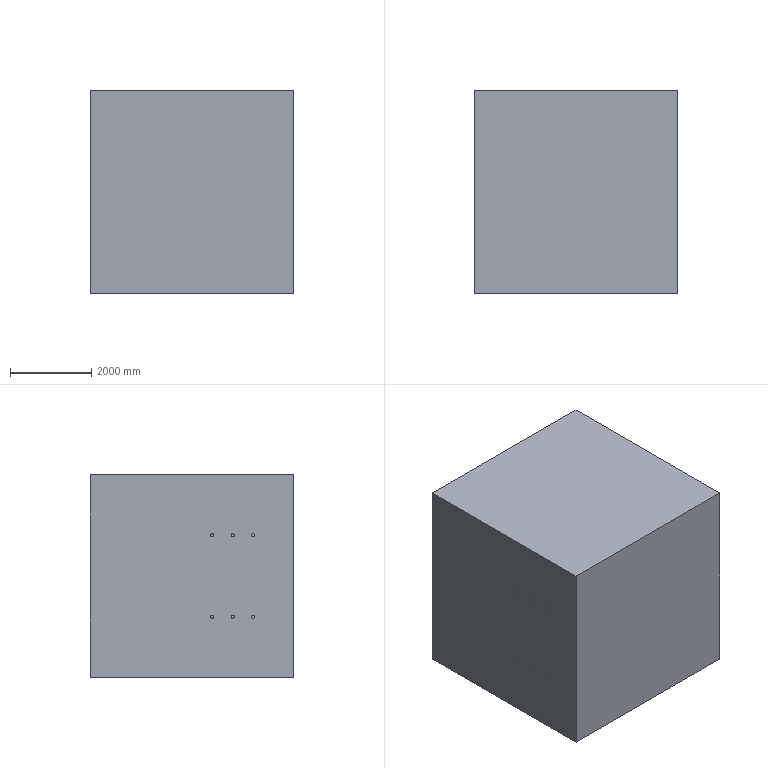Simulation study | ansys fluent
Set-up summary:
category,name,step,type,value,unit,region
solver,ansys_fluent,,Fluent 26.1.0
units,SI m-kg-s (Fluent internal),,stated,boundary values in the units shown in brackets; results in listed units
analysis,deck-1.cas,,"cfd unsteady, 1st-order implicit","dimension=3D; solver=3d, dp, pbns, rke, transient (3d, double precision, pressure-based, realizable k-epsilon, transient); source_case=3.cas.h5"
model,Space,deck-1.cas,,3D
model,Time,deck-1.cas,,"Unsteady, 1st-Order Implicit"
model,Viscous,deck-1.cas,,Realizable k-epsilon turbulence model
model,Wall Treatment,deck-1.cas,,Enhanced Wall Treatment
model,Heat Transfer,deck-1.cas,,Enabled
model,Radiation,deck-1.cas,,Discrete Ordinate Model
model,Multiphase,deck-1.cas,,Disabled
analysis,deck-2.cas,,cfd steady,"dimension=3D; solver=3d, dp, pbns, rke (3d, double precision, pressure-based, realizable k-epsilon); source_case=5.cas.h5"
model,Space,deck-2.cas,,3D
model,Time,deck-2.cas,,Steady
model,Viscous,deck-2.cas,,Realizable k-epsilon turbulence model
model,Wall Treatment,deck-2.cas,,Enhanced Wall Treatment
model,Heat Transfer,deck-2.cas,,Enabled
model,Radiation,deck-2.cas,,Discrete Ordinate Model
model,Multiphase,deck-2.cas,,Disabled
analysis,deck-3.cas,,"cfd unsteady, 1st-order implicit","dimension=3D; solver=3d, dp, pbns, rke, transient (3d, double precision, pressure-based, realizable k-epsilon, transient); source_case=.cas.h5"
model,Space,deck-3.cas,,3D
model,Time,deck-3.cas,,"Unsteady, 1st-Order Implicit"
model,Viscous,deck-3.cas,,Realizable k-epsilon turbulence model
model,Wall Treatment,deck-3.cas,,Enhanced Wall Treatment
model,Heat Transfer,deck-3.cas,,Enabled
model,Radiation,deck-3.cas,,Discrete Ordinate Model
model,Multiphase,deck-3.cas,,Disabled
mesh,deck-1.cas,,nodes,600032
mesh,deck-1.cas,,elements,146215
mesh,deck-1.cas,,faces,826216
mesh,deck-1.cas,,note,elements = cells; counts from the case file zone headers
mesh,deck-2.cas,,nodes,600032
mesh,deck-2.cas,,elements,146215
mesh,deck-2.cas,,faces,826216
mesh,deck-2.cas,,note,elements = cells; counts from the case file zone headers
mesh,deck-3.cas,,nodes,600032
mesh,deck-3.cas,,elements,146215
mesh,deck-3.cas,,faces,826216
mesh,deck-3.cas,,note,elements = cells; counts from the case file zone headers
cell_zone,dead0,deck-1.cas,solid,material=zhujian,,zone 499
cell_zone,room,deck-1.cas,fluid,material=air,,zone 496
cell_zone,dead0,deck-2.cas,solid,material=zhujian,,zone 499
cell_zone,room,deck-2.cas,fluid,material=air,,zone 496
cell_zone,dead0,deck-3.cas,solid,material=zhujian,,zone 499
cell_zone,room,deck-3.cas,fluid,material=air,,zone 496
material,zhujian (solid),,Density,7200,kg/m^3
material,zhujian (solid),,Cp (Specific Heat),540,J/(kg K)
material,zhujian (solid),,Thermal Conductivity,45,W/(m K)
material,zhujian (solid),,Absorption Coefficient,0,m^-1
material,zhujian (solid),,Scattering Coefficient,0,m^-1
material,zhujian (solid),,Scattering Phase Function,isotropic: #f
material,zhujian (solid),,Refractive Index,1
material,steel (solid),,Density,8030,kg/m^3
material,steel (solid),,Cp (Specific Heat),502.48,J/(kg K)
material,steel (solid),,Thermal Conductivity,16.27,W/(m K)
material,steel (solid),,Absorption Coefficient,0,m^-1
material,steel (solid),,Scattering Coefficient,0,m^-1
material,steel (solid),,Scattering Phase Function,isotropic: #f
material,steel (solid),,Refractive Index,1
material,air (fluid),,Density,1.06,kg/m^3
material,air (fluid),,Cp (Specific Heat),1009,J/(kg K)
material,air (fluid),,Thermal Conductivity,0.029,W/(m K)
material,air (fluid),,Viscosity,2.05e-05,kg/(m s)
material,air (fluid),,Absorption Coefficient,0,m^-1
material,air (fluid),,Scattering Coefficient,0,m^-1
material,air (fluid),,Scattering Phase Function,isotropic: #f
material,air (fluid),,Refractive Index,1
bc,bot,deck-1.cas,wall,Material Name=steel; Thermal BC Type=Heat Flux; Wall Motion=Stationary Wall; Shear Boundary Condition=No Slip,,zone 31
bc,wall-fushe,deck-1.cas,wall,Material Name=steel; Thermal BC Type=Temperature; Temperature [C]=30; Wall Motion=Stationary Wall; Shear Boundary Condition=No Slip; Internal Emissivity=0.85,,zone 27
bc,top,deck-1.cas,wall,Material Name=steel; Thermal BC Type=Heat Flux; Wall Motion=Stationary Wall; Shear Boundary Condition=No Slip,,zone 32
bc,room:1,deck-1.cas,wall,Material Name=steel; Thermal BC Type=Heat Flux; Wall Motion=Stationary Wall; Shear Boundary Condition=No Slip,,zone 26
bc,wall-zhujian,deck-1.cas,wall,Material Name=zhujian; Thermal BC Type=Coupled; Wall Motion=Stationary Wall; Shear Boundary Condition=No Slip; Internal Emissivity=0.85,,zone 30
bc,outlet,deck-1.cas,pressure-outlet,,,zone 29
bc,inlet,deck-1.cas,velocity-inlet,Velocity Magnitude [m/s]=20; Temperature [C]=20; Turbulence Specification Method=Intensity and Hydraulic Diameter; Hydraulic Diameter [mm]=80,,zone 28
bc,wall-zhujian-shadow,deck-1.cas,wall,Material Name=zhujian; Thermal BC Type=Coupled,,zone 2
bc,bot,deck-2.cas,wall,Material Name=steel; Thermal BC Type=Heat Flux; Wall Motion=Stationary Wall; Shear Boundary Condition=No Slip,,zone 31
bc,wall-fushe,deck-2.cas,wall,Material Name=steel; Thermal BC Type=Temperature; Temperature [C]=30; Wall Motion=Stationary Wall; Shear Boundary Condition=No Slip; Internal Emissivity=0.85,,zone 27
bc,top,deck-2.cas,wall,Material Name=steel; Thermal BC Type=Heat Flux; Wall Motion=Stationary Wall; Shear Boundary Condition=No Slip,,zone 32
bc,room:1,deck-2.cas,wall,Material Name=steel; Thermal BC Type=Heat Flux; Wall Motion=Stationary Wall; Shear Boundary Condition=No Slip,,zone 26
bc,wall-zhujian,deck-2.cas,wall,Material Name=zhujian; Thermal BC Type=Coupled; Wall Motion=Stationary Wall; Shear Boundary Condition=No Slip; Internal Emissivity=0.85,,zone 30
bc,outlet,deck-2.cas,pressure-outlet,,,zone 29
bc,inlet,deck-2.cas,velocity-inlet,Velocity Magnitude [m/s]=20; Temperature [C]=20; Turbulence Specification Method=Intensity and Hydraulic Diameter; Hydraulic Diameter [mm]=80,,zone 28
bc,wall-zhujian-shadow,deck-2.cas,wall,Material Name=zhujian; Thermal BC Type=Coupled,,zone 2
bc,bot,deck-3.cas,wall,Material Name=steel; Thermal BC Type=Heat Flux; Wall Motion=Stationary Wall; Shear Boundary Condition=No Slip,,zone 31
bc,wall-fushe,deck-3.cas,wall,Material Name=steel; Thermal BC Type=Temperature; Temperature [C]=30; Wall Motion=Stationary Wall; Shear Boundary Condition=No Slip; Internal Emissivity=0.85,,zone 27
bc,top,deck-3.cas,wall,Material Name=steel; Thermal BC Type=Heat Flux; Wall Motion=Stationary Wall; Shear Boundary Condition=No Slip,,zone 32
bc,room:1,deck-3.cas,wall,Material Name=steel; Thermal BC Type=Heat Flux; Wall Motion=Stationary Wall; Shear Boundary Condition=No Slip,,zone 26
bc,wall-zhujian,deck-3.cas,wall,Material Name=zhujian; Thermal BC Type=Coupled; Wall Motion=Stationary Wall; Shear Boundary Condition=No Slip; Internal Emissivity=0.85,,zone 30
bc,outlet,deck-3.cas,pressure-outlet,,,zone 29
bc,inlet,deck-3.cas,velocity-inlet,Velocity Magnitude [m/s]=20; Temperature [C]=20; Turbulence Specification Method=Intensity and Hydraulic Diameter; Hydraulic Diameter [mm]=80,,zone 28
bc,wall-zhujian-shadow,deck-3.cas,wall,Material Name=zhujian; Thermal BC Type=Coupled,,zone 2
Results summary, first 58 of 117 lines:
result,mass flow rate bot,deck-1.cas,,-0,kg/s
result,mass flow rate inlet,deck-1.cas,,0.6277,kg/s
result,mass flow rate outlet,deck-1.cas,,-0.6281,kg/s
result,mass flow rate room:1,deck-1.cas,,-0,kg/s
result,mass flow rate top,deck-1.cas,,-0,kg/s
result,mass flow rate wall-fushe,deck-1.cas,,-0,kg/s
result,mass flow rate wall-zhujian,deck-1.cas,,-0,kg/s
result,mass flow rate wall-zhujian-shadow,deck-1.cas,,-0,kg/s
result,mass flow rate Net,deck-1.cas,,-0.0004064,kg/s
result,heat transfer rate bot,deck-1.cas,,-0,W
result,heat transfer rate inlet,deck-1.cas,,-3195.02,W
result,heat transfer rate outlet,deck-1.cas,,-39657.9,W
result,heat transfer rate room:1,deck-1.cas,,-0,W
result,heat transfer rate top,deck-1.cas,,-0,W
result,heat transfer rate wall-fushe,deck-1.cas,,-9096,W
result,heat transfer rate wall-zhujian,deck-1.cas,,50673.9,W
result,heat transfer rate wall-zhujian-shadow,deck-1.cas,,-50673.9,W
result,heat transfer rate Net,deck-1.cas,,-51948.9,W
result,wall force total bot,deck-1.cas,,"(0.01682, -483.115, -0.0206)",N
result,wall force pressure bot,deck-1.cas,,"(0, -483.115, 0)",N
result,wall force viscous bot,deck-1.cas,,"(0.01682, 0, -0.0206)",N
result,wall force total room:1,deck-1.cas,,"(0.4087, 0.04633, 0.1506)",N
result,wall force pressure room:1,deck-1.cas,,"(0.3535, 1.20603e-14, 0.2096)",N
result,wall force viscous room:1,deck-1.cas,,"(0.05521, 0.04633, -0.05892)",N
result,wall force total top,deck-1.cas,,"(0.01056, 285.279, 0.0005891)",N
result,wall force pressure top,deck-1.cas,,"(-6.71006e-15, 285.279, -1.05796e-14)",N
result,wall force viscous top,deck-1.cas,,"(0.01056, -1.11714e-19, 0.0005891)",N
result,wall force total wall-fushe,deck-1.cas,,"(0.005408, 197.691, 0.0007504)",N
result,wall force pressure wall-fushe,deck-1.cas,,"(-6.43113e-15, 197.691, 1.0544e-14)",N
result,wall force viscous wall-fushe,deck-1.cas,,"(0.005408, 8.03765e-20, 0.0007504)",N
result,wall force total wall-zhujian,deck-1.cas,,"(9.413, 0.02915, -0.3709)",N
result,wall force pressure wall-zhujian,deck-1.cas,,"(9.414, 0.07882, -0.2936)",N
result,wall force viscous wall-zhujian,deck-1.cas,,"(-0.0006776, -0.04968, -0.07731)",N
result,wall force total wall-zhujian-shadow,deck-1.cas,,"(0, 0, 0)",N
result,wall force pressure wall-zhujian-shadow,deck-1.cas,,"(0, 0, 0)",N
result,wall force viscous wall-zhujian-shadow,deck-1.cas,,"(0, 0, 0)",N
result,wall force total Net,deck-1.cas,,"(9.855, -0.06937, -0.2395)",N
result,wall force pressure Net,deck-1.cas,,"(9.767, -0.06603, -0.08402)",N
result,wall force viscous Net,deck-1.cas,,"(0.08732, -0.003349, -0.1555)",N
result,mass flow rate bot,deck-2.cas,,-0,kg/s
result,mass flow rate inlet,deck-2.cas,,0.6277,kg/s
result,mass flow rate outlet,deck-2.cas,,-0.6281,kg/s
result,mass flow rate room:1,deck-2.cas,,-0,kg/s
result,mass flow rate top,deck-2.cas,,-0,kg/s
result,mass flow rate wall-fushe,deck-2.cas,,-0,kg/s
result,mass flow rate wall-zhujian,deck-2.cas,,-0,kg/s
result,mass flow rate wall-zhujian-shadow,deck-2.cas,,-0,kg/s
result,mass flow rate Net,deck-2.cas,,-0.0004064,kg/s
result,heat transfer rate bot,deck-2.cas,,-0,W
result,heat transfer rate inlet,deck-2.cas,,-0,W
result,heat transfer rate outlet,deck-2.cas,,-0,W
result,heat transfer rate room:1,deck-2.cas,,-0,W
result,heat transfer rate top,deck-2.cas,,-0,W
result,heat transfer rate wall-fushe,deck-2.cas,,-0,W
result,heat transfer rate wall-zhujian,deck-2.cas,,-0,W
result,heat transfer rate wall-zhujian-shadow,deck-2.cas,,-0,W
result,heat transfer rate Net,deck-2.cas,,0,W
result,wall force total bot,deck-2.cas,,"(0.01682, -483.115, -0.0206)",N